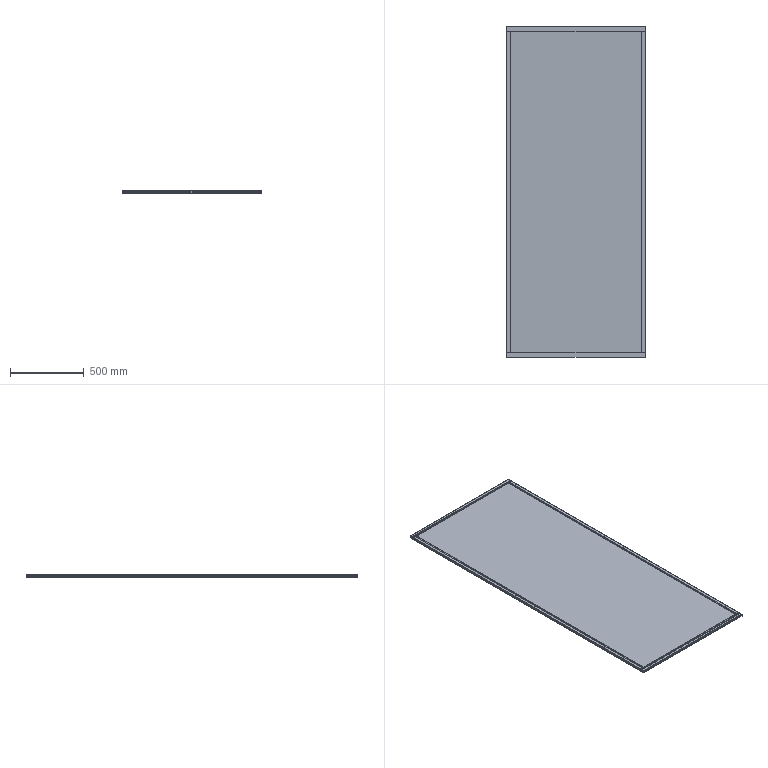Part | SolidWorks | features ICE 2, WeldMemberFeat 1, WeldmentFeature 1 | 5 solids | 167 faces | box 940 x 2236 x 18 mm | volume 20877924 mm3 | plane 98 | cylinder 69 | commonest cylinder face diameters 1.1 x24 3.6 x20 5.8 x20 1 x5